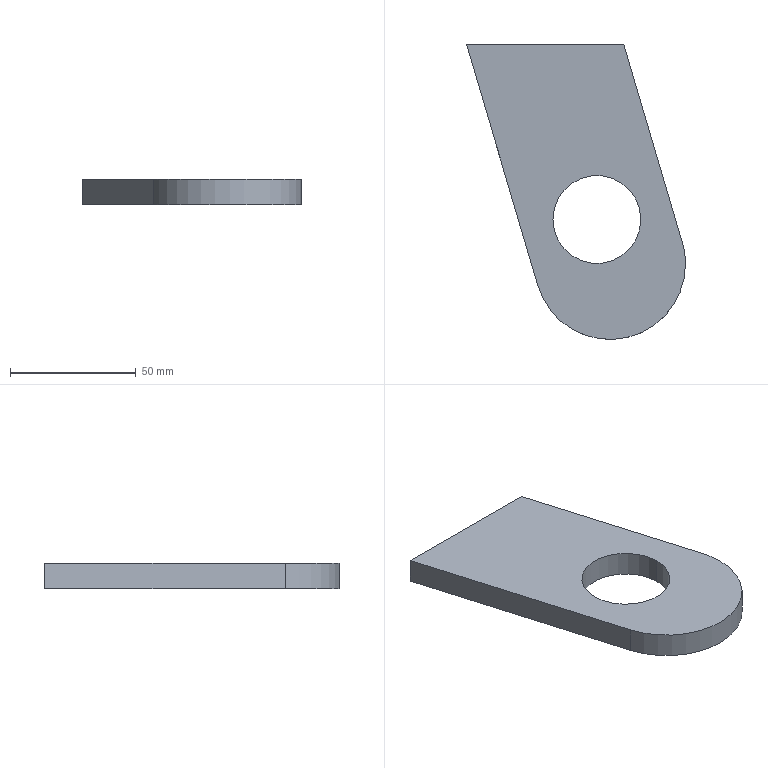Part | SolidWorks | features Extrusion 1 | 1 solid | 9 faces | box 87.114 x 117.396 x 10 mm | volume 59196 mm3 | plane 5 | cylinder 4 | commonest cylinder face diameters 35 x2 60 x2
STEP:
#1=CARTESIAN_POINT('',(541.428,-291.752,-10.));
#2=VERTEX_POINT('',#1);
#3=CARTESIAN_POINT('',(576.428,-291.752,-10.));
#4=VERTEX_POINT('',#3);
#5=CARTESIAN_POINT('',(558.928,-291.752,-10.));
#6=DIRECTION('',(0.,0.,1.));
#7=DIRECTION('',(1.,0.,0.));
#8=AXIS2_PLACEMENT_3D('',#5,#6,#7);
#9=CIRCLE('',#8,17.5);
#10=EDGE_CURVE('',#2,#4,#9,.T.);
#11=ORIENTED_EDGE('',*,*,#10,.F.);
#12=CARTESIAN_POINT('',(541.428,-291.752,0.));
#13=VERTEX_POINT('',#12);
#14=CARTESIAN_POINT('',(541.428,-291.752,-10.));
#15=DIRECTION('',(0.,0.,1.));
#16=VECTOR('',#15,1000.);
#17=LINE('',#14,#16);
#18=EDGE_CURVE('',#2,#13,#17,.T.);
#19=ORIENTED_EDGE('',*,*,#18,.T.);
#20=CARTESIAN_POINT('',(576.428,-291.752,0.));
#21=VERTEX_POINT('',#20);
#22=CARTESIAN_POINT('',(558.928,-291.752,0.));
#23=DIRECTION('',(0.,0.,1.));
#24=DIRECTION('',(1.,0.,0.));
#25=AXIS2_PLACEMENT_3D('',#22,#23,#24);
#26=CIRCLE('',#25,17.5);
#27=EDGE_CURVE('',#13,#21,#26,.T.);
#28=ORIENTED_EDGE('',*,*,#27,.T.);
#29=CARTESIAN_POINT('',(576.428,-291.752,-10.));
#30=DIRECTION('',(0.,0.,1.));
#31=VECTOR('',#30,1000.);
#32=LINE('',#29,#31);
#33=EDGE_CURVE('',#4,#21,#32,.T.);
#34=ORIENTED_EDGE('',*,*,#33,.F.);
#35=EDGE_LOOP('',(#11,#19,#28,#34));
#36=FACE_OUTER_BOUND('',#35,.T.);
#37=CARTESIAN_POINT('',(558.928,-291.752,-10.));
#38=DIRECTION('',(0.,0.,1.));
#39=DIRECTION('',(1.,0.,0.));
#40=AXIS2_PLACEMENT_3D('',#37,#38,#39);
#41=CYLINDRICAL_SURFACE('',#40,17.5);
#42=ADVANCED_FACE('',(#36),#41,.F.);
#43=CARTESIAN_POINT('',(535.409,-318.022,-10.));
#44=VERTEX_POINT('',#43);
#45=CARTESIAN_POINT('',(594.179,-309.519,-10.));
#46=VERTEX_POINT('',#45);
#47=CARTESIAN_POINT('',(564.179,-309.519,-10.));
#48=DIRECTION('',(0.,0.,1.));
#49=DIRECTION('',(1.,0.,0.));
#50=AXIS2_PLACEMENT_3D('',#47,#48,#49);
#51=CIRCLE('',#50,30.);
#52=EDGE_CURVE('',#44,#46,#51,.T.);
#53=ORIENTED_EDGE('',*,*,#52,.T.);
#54=CARTESIAN_POINT('',(594.179,-309.519,0.));
#55=VERTEX_POINT('',#54);
#56=CARTESIAN_POINT('',(594.179,-309.519,-10.));
#57=DIRECTION('',(0.,0.,1.));
#58=VECTOR('',#57,1000.);
#59=LINE('',#56,#58);
#60=EDGE_CURVE('',#46,#55,#59,.T.);
#61=ORIENTED_EDGE('',*,*,#60,.T.);
#62=CARTESIAN_POINT('',(535.409,-318.022,0.));
#63=VERTEX_POINT('',#62);
#64=CARTESIAN_POINT('',(564.179,-309.519,0.));
#65=DIRECTION('',(0.,0.,1.));
#66=DIRECTION('',(1.,0.,0.));
#67=AXIS2_PLACEMENT_3D('',#64,#65,#66);
#68=CIRCLE('',#67,30.);
#69=EDGE_CURVE('',#63,#55,#68,.T.);
#70=ORIENTED_EDGE('',*,*,#69,.F.);
#71=CARTESIAN_POINT('',(535.409,-318.022,-10.));
#72=DIRECTION('',(0.,0.,1.));
#73=VECTOR('',#72,1000.);
#74=LINE('',#71,#73);
#75=EDGE_CURVE('',#44,#63,#74,.T.);
#76=ORIENTED_EDGE('',*,*,#75,.F.);
#77=EDGE_LOOP('',(#53,#61,#70,#76));
#78=FACE_OUTER_BOUND('',#77,.T.);
#79=CARTESIAN_POINT('',(564.179,-309.519,-10.));
#80=DIRECTION('',(0.,0.,1.));
#81=DIRECTION('',(1.,0.,0.));
#82=AXIS2_PLACEMENT_3D('',#79,#80,#81);
#83=CYLINDRICAL_SURFACE('',#82,30.);
#84=ADVANCED_FACE('',(#78),#83,.T.);
#85=CARTESIAN_POINT('',(569.631,-222.123,0.));
#86=VERTEX_POINT('',#85);
#87=CARTESIAN_POINT('',(507.065,-222.123,0.));
#88=VERTEX_POINT('',#87);
#89=CARTESIAN_POINT('',(507.065,-222.123,0.));
#90=DIRECTION('',(-1.,0.,0.));
#91=VECTOR('',#90,1000.);
#92=LINE('',#89,#91);
#93=EDGE_CURVE('',#86,#88,#92,.T.);
#94=ORIENTED_EDGE('',*,*,#93,.F.);
#95=CARTESIAN_POINT('',(569.631,-222.123,-10.));
#96=VERTEX_POINT('',#95);
#97=CARTESIAN_POINT('',(569.631,-222.123,-10.));
#98=DIRECTION('',(0.,0.,1.));
#99=VECTOR('',#98,1000.);
#100=LINE('',#97,#99);
#101=EDGE_CURVE('',#96,#86,#100,.T.);
#102=ORIENTED_EDGE('',*,*,#101,.F.);
#103=CARTESIAN_POINT('',(507.065,-222.123,-10.));
#104=VERTEX_POINT('',#103);
#105=CARTESIAN_POINT('',(507.065,-222.123,-10.));
#106=DIRECTION('',(-1.,0.,0.));
#107=VECTOR('',#106,1000.);
#108=LINE('',#105,#107);
#109=EDGE_CURVE('',#96,#104,#108,.T.);
#110=ORIENTED_EDGE('',*,*,#109,.T.);
#111=CARTESIAN_POINT('',(507.065,-222.123,-10.));
#112=DIRECTION('',(0.,0.,1.));
#113=VECTOR('',#112,1000.);
#114=LINE('',#111,#113);
#115=EDGE_CURVE('',#104,#88,#114,.T.);
#116=ORIENTED_EDGE('',*,*,#115,.T.);
#117=EDGE_LOOP('',(#94,#102,#110,#116));
#118=FACE_OUTER_BOUND('',#117,.T.);
#119=CARTESIAN_POINT('',(507.065,-222.123,-10.));
#120=DIRECTION('',(0.,1.,0.));
#121=DIRECTION('',(0.,0.,1.));
#122=AXIS2_PLACEMENT_3D('',#119,#120,#121);
#123=PLANE('',#122);
#124=ADVANCED_FACE('',(#118),#123,.T.);
#125=CARTESIAN_POINT('',(592.949,-301.015,0.));
#126=VERTEX_POINT('',#125);
#127=CARTESIAN_POINT('',(569.631,-222.123,0.));
#128=DIRECTION('',(-0.2834,0.959,0.));
#129=VECTOR('',#128,1000.);
#130=LINE('',#127,#129);
#131=EDGE_CURVE('',#126,#86,#130,.T.);
#132=ORIENTED_EDGE('',*,*,#131,.F.);
#133=CARTESIAN_POINT('',(592.949,-301.015,-10.));
#134=VERTEX_POINT('',#133);
#135=CARTESIAN_POINT('',(592.949,-301.015,-10.));
#136=DIRECTION('',(0.,0.,1.));
#137=VECTOR('',#136,1000.);
#138=LINE('',#135,#137);
#139=EDGE_CURVE('',#134,#126,#138,.T.);
#140=ORIENTED_EDGE('',*,*,#139,.F.);
#141=CARTESIAN_POINT('',(569.631,-222.123,-10.));
#142=DIRECTION('',(-0.2834,0.959,0.));
#143=VECTOR('',#142,1000.);
#144=LINE('',#141,#143);
#145=EDGE_CURVE('',#134,#96,#144,.T.);
#146=ORIENTED_EDGE('',*,*,#145,.T.);
#147=ORIENTED_EDGE('',*,*,#101,.T.);
#148=EDGE_LOOP('',(#132,#140,#146,#147));
#149=FACE_OUTER_BOUND('',#148,.T.);
#150=CARTESIAN_POINT('',(569.631,-222.123,-10.));
#151=DIRECTION('',(0.959,0.2834,0.));
#152=DIRECTION('',(-0.2834,0.959,0.));
#153=AXIS2_PLACEMENT_3D('',#150,#151,#152);
#154=PLANE('',#153);
#155=ADVANCED_FACE('',(#149),#154,.T.);
#156=ORIENTED_EDGE('',*,*,#60,.F.);
#157=CARTESIAN_POINT('',(564.179,-309.519,-10.));
#158=DIRECTION('',(0.,0.,1.));
#159=DIRECTION('',(1.,0.,0.));
#160=AXIS2_PLACEMENT_3D('',#157,#158,#159);
#161=CIRCLE('',#160,30.);
#162=EDGE_CURVE('',#46,#134,#161,.T.);
#163=ORIENTED_EDGE('',*,*,#162,.T.);
#164=ORIENTED_EDGE('',*,*,#139,.T.);
#165=CARTESIAN_POINT('',(564.179,-309.519,0.));
#166=DIRECTION('',(0.,0.,1.));
#167=DIRECTION('',(1.,0.,0.));
#168=AXIS2_PLACEMENT_3D('',#165,#166,#167);
#169=CIRCLE('',#168,30.);
#170=EDGE_CURVE('',#55,#126,#169,.T.);
#171=ORIENTED_EDGE('',*,*,#170,.F.);
#172=EDGE_LOOP('',(#156,#163,#164,#171));
#173=FACE_OUTER_BOUND('',#172,.T.);
#174=CARTESIAN_POINT('',(564.179,-309.519,-10.));
#175=DIRECTION('',(0.,0.,1.));
#176=DIRECTION('',(1.,0.,0.));
#177=AXIS2_PLACEMENT_3D('',#174,#175,#176);
#178=CYLINDRICAL_SURFACE('',#177,30.);
#179=ADVANCED_FACE('',(#173),#178,.T.);
#180=CARTESIAN_POINT('',(507.065,-222.123,0.));
#181=DIRECTION('',(0.2834,-0.959,0.));
#182=VECTOR('',#181,1000.);
#183=LINE('',#180,#182);
#184=EDGE_CURVE('',#88,#63,#183,.T.);
#185=ORIENTED_EDGE('',*,*,#184,.F.);
#186=ORIENTED_EDGE('',*,*,#115,.F.);
#187=CARTESIAN_POINT('',(507.065,-222.123,-10.));
#188=DIRECTION('',(0.2834,-0.959,0.));
#189=VECTOR('',#188,1000.);
#190=LINE('',#187,#189);
#191=EDGE_CURVE('',#104,#44,#190,.T.);
#192=ORIENTED_EDGE('',*,*,#191,.T.);
#193=ORIENTED_EDGE('',*,*,#75,.T.);
#194=EDGE_LOOP('',(#185,#186,#192,#193));
#195=FACE_OUTER_BOUND('',#194,.T.);
#196=CARTESIAN_POINT('',(507.065,-222.123,-10.));
#197=DIRECTION('',(-0.959,-0.2834,0.));
#198=DIRECTION('',(0.2834,-0.959,0.));
#199=AXIS2_PLACEMENT_3D('',#196,#197,#198);
#200=PLANE('',#199);
#201=ADVANCED_FACE('',(#195),#200,.T.);
#202=CARTESIAN_POINT('',(558.928,-291.752,-10.));
#203=DIRECTION('',(0.,0.,1.));
#204=DIRECTION('',(1.,0.,0.));
#205=AXIS2_PLACEMENT_3D('',#202,#203,#204);
#206=CIRCLE('',#205,17.5);
#207=EDGE_CURVE('',#4,#2,#206,.T.);
#208=ORIENTED_EDGE('',*,*,#207,.T.);
#209=ORIENTED_EDGE('',*,*,#10,.T.);
#210=EDGE_LOOP('',(#208,#209));
#211=FACE_BOUND('',#210,.T.);
#212=ORIENTED_EDGE('',*,*,#109,.F.);
#213=ORIENTED_EDGE('',*,*,#145,.F.);
#214=ORIENTED_EDGE('',*,*,#162,.F.);
#215=ORIENTED_EDGE('',*,*,#52,.F.);
#216=ORIENTED_EDGE('',*,*,#191,.F.);
#217=EDGE_LOOP('',(#212,#213,#214,#215,#216));
#218=FACE_OUTER_BOUND('',#217,.T.);
#219=CARTESIAN_POINT('',(564.179,-309.519,-10.));
#220=DIRECTION('',(0.,0.,1.));
#221=DIRECTION('',(1.,0.,0.));
#222=AXIS2_PLACEMENT_3D('',#219,#220,#221);
#223=PLANE('',#222);
#224=ADVANCED_FACE('',(#211,#218),#223,.F.);
#225=CARTESIAN_POINT('',(558.928,-291.752,0.));
#226=DIRECTION('',(0.,0.,1.));
#227=DIRECTION('',(1.,0.,0.));
#228=AXIS2_PLACEMENT_3D('',#225,#226,#227);
#229=CIRCLE('',#228,17.5);
#230=EDGE_CURVE('',#21,#13,#229,.T.);
#231=ORIENTED_EDGE('',*,*,#230,.F.);
#232=ORIENTED_EDGE('',*,*,#27,.F.);
#233=EDGE_LOOP('',(#231,#232));
#234=FACE_BOUND('',#233,.T.);
#235=ORIENTED_EDGE('',*,*,#93,.T.);
#236=ORIENTED_EDGE('',*,*,#184,.T.);
#237=ORIENTED_EDGE('',*,*,#69,.T.);
#238=ORIENTED_EDGE('',*,*,#170,.T.);
#239=ORIENTED_EDGE('',*,*,#131,.T.);
#240=EDGE_LOOP('',(#235,#236,#237,#238,#239));
#241=FACE_OUTER_BOUND('',#240,.T.);
#242=CARTESIAN_POINT('',(564.179,-309.519,0.));
#243=DIRECTION('',(0.,0.,1.));
#244=DIRECTION('',(1.,0.,0.));
#245=AXIS2_PLACEMENT_3D('',#242,#243,#244);
#246=PLANE('',#245);
#247=ADVANCED_FACE('',(#234,#241),#246,.T.);
#248=ORIENTED_EDGE('',*,*,#18,.F.);
#249=ORIENTED_EDGE('',*,*,#207,.F.);
#250=ORIENTED_EDGE('',*,*,#33,.T.);
#251=ORIENTED_EDGE('',*,*,#230,.T.);
#252=EDGE_LOOP('',(#248,#249,#250,#251));
#253=FACE_OUTER_BOUND('',#252,.T.);
#254=CARTESIAN_POINT('',(558.928,-291.752,-10.));
#255=DIRECTION('',(0.,0.,1.));
#256=DIRECTION('',(1.,0.,0.));
#257=AXIS2_PLACEMENT_3D('',#254,#255,#256);
#258=CYLINDRICAL_SURFACE('',#257,17.5);
#259=ADVANCED_FACE('',(#253),#258,.F.);
#260=CLOSED_SHELL('',(#42,#84,#124,#155,#179,#201,#224,#247,#259));
#261=MANIFOLD_SOLID_BREP('',#260);
#262=CARTESIAN_POINT('',(0.,0.,0.));
#263=DIRECTION('',(0.,0.,1.));
#264=DIRECTION('',(1.,0.,0.));
#265=AXIS2_PLACEMENT_3D('',#262,#263,#264);
#266=(LENGTH_UNIT()NAMED_UNIT(*)SI_UNIT(.MILLI.,.METRE.));
#267=UNCERTAINTY_MEASURE_WITH_UNIT(LENGTH_MEASURE(0.00001),#266,'','');
#268=(NAMED_UNIT(*)PLANE_ANGLE_UNIT()SI_UNIT($,.RADIAN.));
#269=(NAMED_UNIT(*)SI_UNIT($,.STERADIAN.)SOLID_ANGLE_UNIT());
#270=(GEOMETRIC_REPRESENTATION_CONTEXT(3)GLOBAL_UNCERTAINTY_ASSIGNED_CONTEXT((#267))GLOBAL_UNIT_ASSIGNED_CONTEXT((#266,#268,#269))REPRESENTATION_CONTEXT('',''));
#271=ADVANCED_BREP_SHAPE_REPRESENTATION('',(#261,#265),#270);